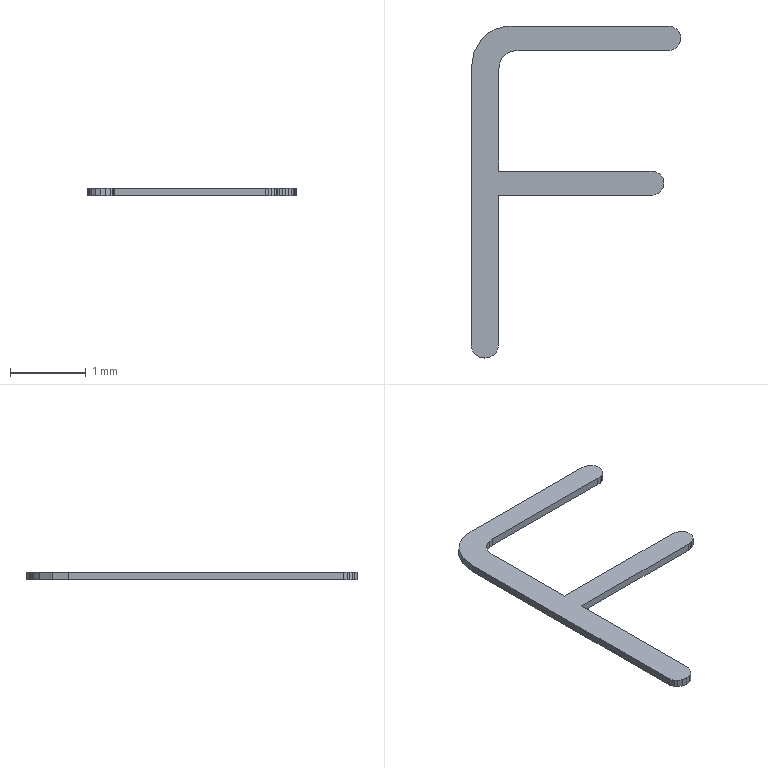Part | STEP file | PART242.stp | 1 solid | 61 faces | box 2.768 x 4.388 x 0.1 mm | volume 0.2981 mm3 | plane 61